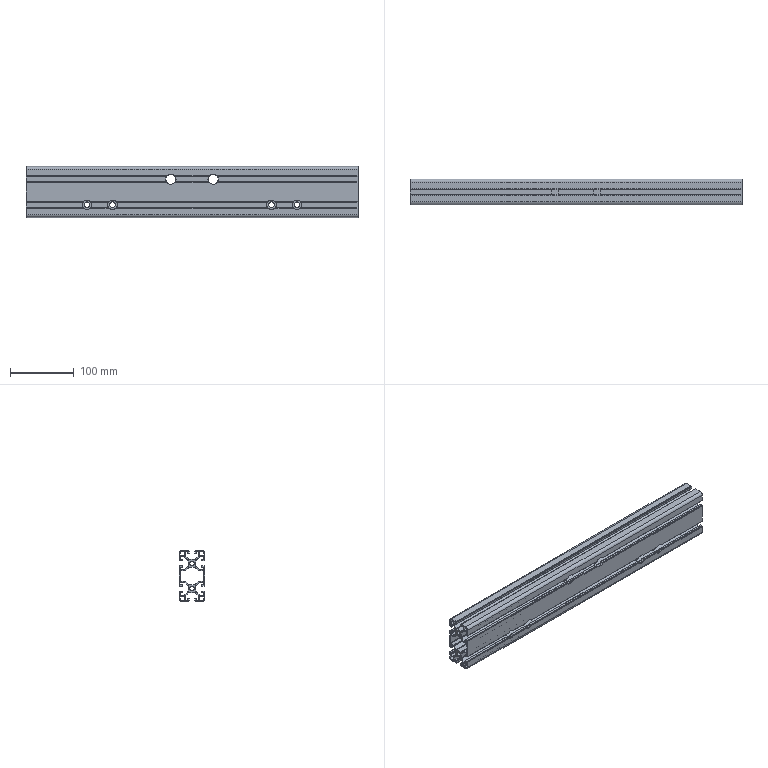Part | STEP file | Fixing rod L520 | 1 solid | 598 faces | box 520 x 40 x 80 mm | volume 414666 mm3 | cylinder 348 | plane 250 | commonest cylinder face diameters 0.6 x112 2 x60 4 x52 0.4 x38 9 x24 15 x20